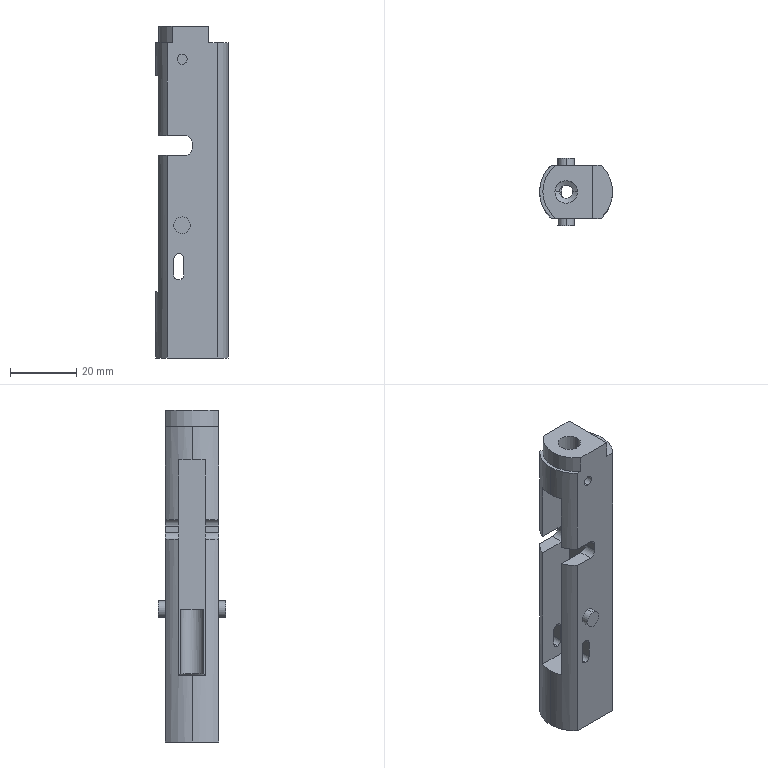Part | SolidWorks | features ICE 11, 3DProfileFeature 2, HoleWzd 2, Extrusion 1, MirrorPattern 1 | 1 solid | 62 faces | box 22 x 20.4 x 100 mm | volume 22225 mm3 | cylinder 31 | plane 27 | cone 4 | commonest cylinder face diameters 3 x10 4 x6 22 x5 5 x4 6.8 x2 10.5 x2